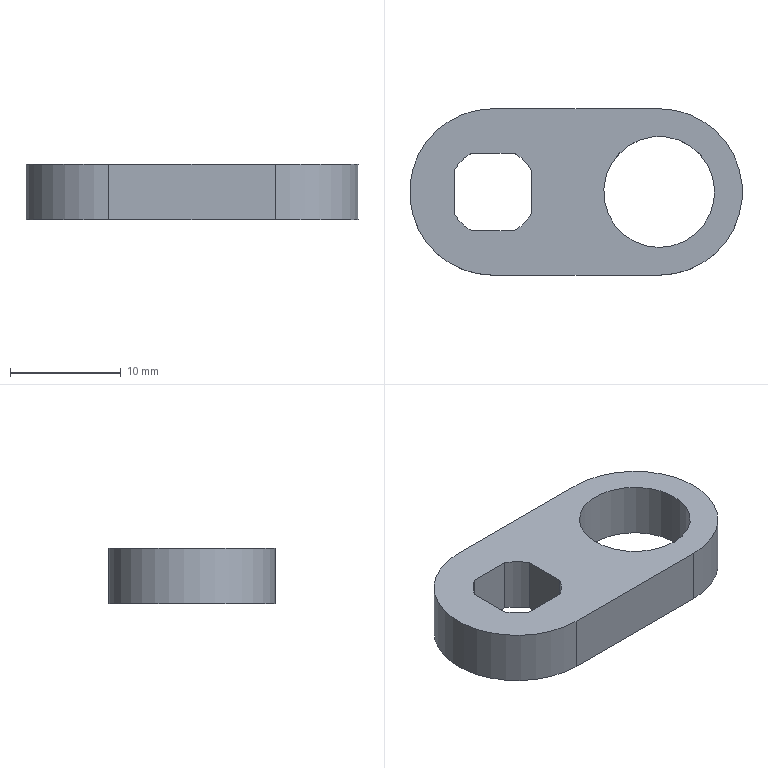Part | NX | features BREP 1, DATUM_CSYS 1 | 1 solid | 15 faces | box 30 x 15 x 5 mm | volume 1391 mm3 | plane 8 | cylinder 7 | commonest cylinder face diameters 8 x4 15 x2 10 x1
STEP:
#1=CARTESIAN_POINT('',(15.,7.5,0.));
#2=VERTEX_POINT('',#1);
#3=CARTESIAN_POINT('',(0.,7.5,0.));
#4=VERTEX_POINT('',#3);
#5=CARTESIAN_POINT('',(15.,7.5,0.));
#6=DIRECTION('',(-1.,0.,0.));
#7=VECTOR('',#6,1000.);
#8=LINE('',#5,#7);
#9=EDGE_CURVE('',#2,#4,#8,.T.);
#10=ORIENTED_EDGE('',*,*,#9,.F.);
#11=CARTESIAN_POINT('',(15.,-7.5,0.));
#12=VERTEX_POINT('',#11);
#13=CARTESIAN_POINT('',(15.,0.,0.));
#14=DIRECTION('',(0.,0.,1.));
#15=DIRECTION('',(0.,-1.,0.));
#16=AXIS2_PLACEMENT_3D('',#13,#14,#15);
#17=CIRCLE('',#16,7.5);
#18=EDGE_CURVE('',#12,#2,#17,.T.);
#19=ORIENTED_EDGE('',*,*,#18,.F.);
#20=CARTESIAN_POINT('',(0.,-7.5,0.));
#21=VERTEX_POINT('',#20);
#22=CARTESIAN_POINT('',(0.,-7.5,0.));
#23=DIRECTION('',(1.,0.,0.));
#24=VECTOR('',#23,1000.);
#25=LINE('',#22,#24);
#26=EDGE_CURVE('',#21,#12,#25,.T.);
#27=ORIENTED_EDGE('',*,*,#26,.F.);
#28=CARTESIAN_POINT('',(0.,0.,0.));
#29=DIRECTION('',(0.,0.,1.));
#30=DIRECTION('',(0.,1.,0.));
#31=AXIS2_PLACEMENT_3D('',#28,#29,#30);
#32=CIRCLE('',#31,7.5);
#33=EDGE_CURVE('',#4,#21,#32,.T.);
#34=ORIENTED_EDGE('',*,*,#33,.F.);
#35=EDGE_LOOP('',(#10,#19,#27,#34));
#36=FACE_BOUND('',#35,.T.);
#37=CARTESIAN_POINT('',(1.936,-3.5,0.));
#38=VERTEX_POINT('',#37);
#39=CARTESIAN_POINT('',(-1.936,-3.5,0.));
#40=VERTEX_POINT('',#39);
#41=CARTESIAN_POINT('',(1.936,-3.5,0.));
#42=DIRECTION('',(-1.,0.,0.));
#43=VECTOR('',#42,1000.);
#44=LINE('',#41,#43);
#45=EDGE_CURVE('',#38,#40,#44,.T.);
#46=ORIENTED_EDGE('',*,*,#45,.F.);
#47=CARTESIAN_POINT('',(3.5,-1.936,0.));
#48=VERTEX_POINT('',#47);
#49=CARTESIAN_POINT('',(0.,0.,0.));
#50=DIRECTION('',(0.,0.,-1.));
#51=DIRECTION('',(0.875,-0.4841,0.));
#52=AXIS2_PLACEMENT_3D('',#49,#50,#51);
#53=CIRCLE('',#52,4.);
#54=EDGE_CURVE('',#48,#38,#53,.T.);
#55=ORIENTED_EDGE('',*,*,#54,.F.);
#56=CARTESIAN_POINT('',(3.5,1.936,0.));
#57=VERTEX_POINT('',#56);
#58=CARTESIAN_POINT('',(3.5,1.936,0.));
#59=DIRECTION('',(0.,-1.,0.));
#60=VECTOR('',#59,1000.);
#61=LINE('',#58,#60);
#62=EDGE_CURVE('',#57,#48,#61,.T.);
#63=ORIENTED_EDGE('',*,*,#62,.F.);
#64=CARTESIAN_POINT('',(1.936,3.5,0.));
#65=VERTEX_POINT('',#64);
#66=CARTESIAN_POINT('',(0.,0.,0.));
#67=DIRECTION('',(0.,0.,-1.));
#68=DIRECTION('',(0.4841,0.875,0.));
#69=AXIS2_PLACEMENT_3D('',#66,#67,#68);
#70=CIRCLE('',#69,4.);
#71=EDGE_CURVE('',#65,#57,#70,.T.);
#72=ORIENTED_EDGE('',*,*,#71,.F.);
#73=CARTESIAN_POINT('',(-1.936,3.5,0.));
#74=VERTEX_POINT('',#73);
#75=CARTESIAN_POINT('',(-1.936,3.5,0.));
#76=DIRECTION('',(1.,0.,0.));
#77=VECTOR('',#76,1000.);
#78=LINE('',#75,#77);
#79=EDGE_CURVE('',#74,#65,#78,.T.);
#80=ORIENTED_EDGE('',*,*,#79,.F.);
#81=CARTESIAN_POINT('',(-3.5,1.936,0.));
#82=VERTEX_POINT('',#81);
#83=CARTESIAN_POINT('',(0.,0.,0.));
#84=DIRECTION('',(0.,0.,-1.));
#85=DIRECTION('',(-0.875,0.4841,0.));
#86=AXIS2_PLACEMENT_3D('',#83,#84,#85);
#87=CIRCLE('',#86,4.);
#88=EDGE_CURVE('',#82,#74,#87,.T.);
#89=ORIENTED_EDGE('',*,*,#88,.F.);
#90=CARTESIAN_POINT('',(-3.5,-1.936,0.));
#91=VERTEX_POINT('',#90);
#92=CARTESIAN_POINT('',(-3.5,-1.936,0.));
#93=DIRECTION('',(0.,1.,0.));
#94=VECTOR('',#93,1000.);
#95=LINE('',#92,#94);
#96=EDGE_CURVE('',#91,#82,#95,.T.);
#97=ORIENTED_EDGE('',*,*,#96,.F.);
#98=CARTESIAN_POINT('',(0.,0.,0.));
#99=DIRECTION('',(0.,0.,-1.));
#100=DIRECTION('',(-0.4841,-0.875,0.));
#101=AXIS2_PLACEMENT_3D('',#98,#99,#100);
#102=CIRCLE('',#101,4.);
#103=EDGE_CURVE('',#40,#91,#102,.T.);
#104=ORIENTED_EDGE('',*,*,#103,.F.);
#105=EDGE_LOOP('',(#46,#55,#63,#72,#80,#89,#97,#104));
#106=FACE_BOUND('',#105,.T.);
#107=CARTESIAN_POINT('',(15.,-5.,0.));
#108=VERTEX_POINT('',#107);
#109=CARTESIAN_POINT('',(15.,0.,0.));
#110=DIRECTION('',(0.,0.,-1.));
#111=DIRECTION('',(0.,-1.,0.));
#112=AXIS2_PLACEMENT_3D('',#109,#110,#111);
#113=CIRCLE('',#112,5.);
#114=EDGE_CURVE('',#108,#108,#113,.T.);
#115=ORIENTED_EDGE('',*,*,#114,.F.);
#116=EDGE_LOOP('',(#115));
#117=FACE_BOUND('',#116,.T.);
#118=CARTESIAN_POINT('',(7.5,7.5,0.));
#119=DIRECTION('',(0.,0.,1.));
#120=DIRECTION('',(-1.,0.,0.));
#121=AXIS2_PLACEMENT_3D('',#118,#119,#120);
#122=PLANE('',#121);
#123=ADVANCED_FACE('',(#36,#106,#117),#122,.F.);
#124=CARTESIAN_POINT('',(0.,7.5,5.));
#125=VERTEX_POINT('',#124);
#126=CARTESIAN_POINT('',(0.,-7.5,5.));
#127=VERTEX_POINT('',#126);
#128=CARTESIAN_POINT('',(0.,0.,5.));
#129=DIRECTION('',(0.,0.,1.));
#130=DIRECTION('',(0.,1.,0.));
#131=AXIS2_PLACEMENT_3D('',#128,#129,#130);
#132=CIRCLE('',#131,7.5);
#133=EDGE_CURVE('',#125,#127,#132,.T.);
#134=ORIENTED_EDGE('',*,*,#133,.T.);
#135=CARTESIAN_POINT('',(15.,-7.5,5.));
#136=VERTEX_POINT('',#135);
#137=CARTESIAN_POINT('',(0.,-7.5,5.));
#138=DIRECTION('',(1.,0.,0.));
#139=VECTOR('',#138,1000.);
#140=LINE('',#137,#139);
#141=EDGE_CURVE('',#127,#136,#140,.T.);
#142=ORIENTED_EDGE('',*,*,#141,.T.);
#143=CARTESIAN_POINT('',(15.,7.5,5.));
#144=VERTEX_POINT('',#143);
#145=CARTESIAN_POINT('',(15.,0.,5.));
#146=DIRECTION('',(0.,0.,1.));
#147=DIRECTION('',(0.,-1.,0.));
#148=AXIS2_PLACEMENT_3D('',#145,#146,#147);
#149=CIRCLE('',#148,7.5);
#150=EDGE_CURVE('',#136,#144,#149,.T.);
#151=ORIENTED_EDGE('',*,*,#150,.T.);
#152=CARTESIAN_POINT('',(15.,7.5,5.));
#153=DIRECTION('',(-1.,0.,0.));
#154=VECTOR('',#153,1000.);
#155=LINE('',#152,#154);
#156=EDGE_CURVE('',#144,#125,#155,.T.);
#157=ORIENTED_EDGE('',*,*,#156,.T.);
#158=EDGE_LOOP('',(#134,#142,#151,#157));
#159=FACE_BOUND('',#158,.T.);
#160=CARTESIAN_POINT('',(-1.936,-3.5,5.));
#161=VERTEX_POINT('',#160);
#162=CARTESIAN_POINT('',(-3.5,-1.936,5.));
#163=VERTEX_POINT('',#162);
#164=CARTESIAN_POINT('',(0.,0.,5.));
#165=DIRECTION('',(0.,0.,-1.));
#166=DIRECTION('',(-0.4841,-0.875,0.));
#167=AXIS2_PLACEMENT_3D('',#164,#165,#166);
#168=CIRCLE('',#167,4.);
#169=EDGE_CURVE('',#161,#163,#168,.T.);
#170=ORIENTED_EDGE('',*,*,#169,.T.);
#171=CARTESIAN_POINT('',(-3.5,1.936,5.));
#172=VERTEX_POINT('',#171);
#173=CARTESIAN_POINT('',(-3.5,-1.936,5.));
#174=DIRECTION('',(0.,1.,0.));
#175=VECTOR('',#174,1000.);
#176=LINE('',#173,#175);
#177=EDGE_CURVE('',#163,#172,#176,.T.);
#178=ORIENTED_EDGE('',*,*,#177,.T.);
#179=CARTESIAN_POINT('',(-1.936,3.5,5.));
#180=VERTEX_POINT('',#179);
#181=CARTESIAN_POINT('',(0.,0.,5.));
#182=DIRECTION('',(0.,0.,-1.));
#183=DIRECTION('',(-0.875,0.4841,0.));
#184=AXIS2_PLACEMENT_3D('',#181,#182,#183);
#185=CIRCLE('',#184,4.);
#186=EDGE_CURVE('',#172,#180,#185,.T.);
#187=ORIENTED_EDGE('',*,*,#186,.T.);
#188=CARTESIAN_POINT('',(1.936,3.5,5.));
#189=VERTEX_POINT('',#188);
#190=CARTESIAN_POINT('',(-1.936,3.5,5.));
#191=DIRECTION('',(1.,0.,0.));
#192=VECTOR('',#191,1000.);
#193=LINE('',#190,#192);
#194=EDGE_CURVE('',#180,#189,#193,.T.);
#195=ORIENTED_EDGE('',*,*,#194,.T.);
#196=CARTESIAN_POINT('',(3.5,1.936,5.));
#197=VERTEX_POINT('',#196);
#198=CARTESIAN_POINT('',(0.,0.,5.));
#199=DIRECTION('',(0.,0.,-1.));
#200=DIRECTION('',(0.4841,0.875,0.));
#201=AXIS2_PLACEMENT_3D('',#198,#199,#200);
#202=CIRCLE('',#201,4.);
#203=EDGE_CURVE('',#189,#197,#202,.T.);
#204=ORIENTED_EDGE('',*,*,#203,.T.);
#205=CARTESIAN_POINT('',(3.5,-1.936,5.));
#206=VERTEX_POINT('',#205);
#207=CARTESIAN_POINT('',(3.5,1.936,5.));
#208=DIRECTION('',(0.,-1.,0.));
#209=VECTOR('',#208,1000.);
#210=LINE('',#207,#209);
#211=EDGE_CURVE('',#197,#206,#210,.T.);
#212=ORIENTED_EDGE('',*,*,#211,.T.);
#213=CARTESIAN_POINT('',(1.936,-3.5,5.));
#214=VERTEX_POINT('',#213);
#215=CARTESIAN_POINT('',(0.,0.,5.));
#216=DIRECTION('',(0.,0.,-1.));
#217=DIRECTION('',(0.875,-0.4841,0.));
#218=AXIS2_PLACEMENT_3D('',#215,#216,#217);
#219=CIRCLE('',#218,4.);
#220=EDGE_CURVE('',#206,#214,#219,.T.);
#221=ORIENTED_EDGE('',*,*,#220,.T.);
#222=CARTESIAN_POINT('',(1.936,-3.5,5.));
#223=DIRECTION('',(-1.,0.,0.));
#224=VECTOR('',#223,1000.);
#225=LINE('',#222,#224);
#226=EDGE_CURVE('',#214,#161,#225,.T.);
#227=ORIENTED_EDGE('',*,*,#226,.T.);
#228=EDGE_LOOP('',(#170,#178,#187,#195,#204,#212,#221,#227));
#229=FACE_BOUND('',#228,.T.);
#230=CARTESIAN_POINT('',(15.,-5.,5.));
#231=VERTEX_POINT('',#230);
#232=CARTESIAN_POINT('',(15.,0.,5.));
#233=DIRECTION('',(0.,0.,-1.));
#234=DIRECTION('',(0.,-1.,0.));
#235=AXIS2_PLACEMENT_3D('',#232,#233,#234);
#236=CIRCLE('',#235,5.);
#237=EDGE_CURVE('',#231,#231,#236,.T.);
#238=ORIENTED_EDGE('',*,*,#237,.T.);
#239=EDGE_LOOP('',(#238));
#240=FACE_BOUND('',#239,.T.);
#241=CARTESIAN_POINT('',(7.5,7.5,5.));
#242=DIRECTION('',(0.,0.,1.));
#243=DIRECTION('',(-1.,0.,0.));
#244=AXIS2_PLACEMENT_3D('',#241,#242,#243);
#245=PLANE('',#244);
#246=ADVANCED_FACE('',(#159,#229,#240),#245,.T.);
#247=ORIENTED_EDGE('',*,*,#33,.T.);
#248=CARTESIAN_POINT('',(0.,-7.5,0.));
#249=DIRECTION('',(0.,0.,1.));
#250=VECTOR('',#249,1000.);
#251=LINE('',#248,#250);
#252=EDGE_CURVE('',#21,#127,#251,.T.);
#253=ORIENTED_EDGE('',*,*,#252,.T.);
#254=ORIENTED_EDGE('',*,*,#133,.F.);
#255=CARTESIAN_POINT('',(0.,7.5,0.));
#256=DIRECTION('',(0.,0.,1.));
#257=VECTOR('',#256,1000.);
#258=LINE('',#255,#257);
#259=EDGE_CURVE('',#4,#125,#258,.T.);
#260=ORIENTED_EDGE('',*,*,#259,.F.);
#261=EDGE_LOOP('',(#247,#253,#254,#260));
#262=FACE_BOUND('',#261,.T.);
#263=CARTESIAN_POINT('',(0.,0.,0.));
#264=DIRECTION('',(0.,0.,1.));
#265=DIRECTION('',(0.,-1.,0.));
#266=AXIS2_PLACEMENT_3D('',#263,#264,#265);
#267=CYLINDRICAL_SURFACE('',#266,7.5);
#268=ADVANCED_FACE('',(#262),#267,.T.);
#269=ORIENTED_EDGE('',*,*,#26,.T.);
#270=CARTESIAN_POINT('',(15.,-7.5,0.));
#271=DIRECTION('',(0.,0.,1.));
#272=VECTOR('',#271,1000.);
#273=LINE('',#270,#272);
#274=EDGE_CURVE('',#12,#136,#273,.T.);
#275=ORIENTED_EDGE('',*,*,#274,.T.);
#276=ORIENTED_EDGE('',*,*,#141,.F.);
#277=ORIENTED_EDGE('',*,*,#252,.F.);
#278=EDGE_LOOP('',(#269,#275,#276,#277));
#279=FACE_BOUND('',#278,.T.);
#280=CARTESIAN_POINT('',(7.5,-7.5,2.5));
#281=DIRECTION('',(0.,-1.,0.));
#282=DIRECTION('',(-1.,0.,0.));
#283=AXIS2_PLACEMENT_3D('',#280,#281,#282);
#284=PLANE('',#283);
#285=ADVANCED_FACE('',(#279),#284,.T.);
#286=ORIENTED_EDGE('',*,*,#18,.T.);
#287=CARTESIAN_POINT('',(15.,7.5,0.));
#288=DIRECTION('',(0.,0.,1.));
#289=VECTOR('',#288,1000.);
#290=LINE('',#287,#289);
#291=EDGE_CURVE('',#2,#144,#290,.T.);
#292=ORIENTED_EDGE('',*,*,#291,.T.);
#293=ORIENTED_EDGE('',*,*,#150,.F.);
#294=ORIENTED_EDGE('',*,*,#274,.F.);
#295=EDGE_LOOP('',(#286,#292,#293,#294));
#296=FACE_BOUND('',#295,.T.);
#297=CARTESIAN_POINT('',(15.,0.,0.));
#298=DIRECTION('',(0.,0.,1.));
#299=DIRECTION('',(0.,1.,0.));
#300=AXIS2_PLACEMENT_3D('',#297,#298,#299);
#301=CYLINDRICAL_SURFACE('',#300,7.5);
#302=ADVANCED_FACE('',(#296),#301,.T.);
#303=ORIENTED_EDGE('',*,*,#9,.T.);
#304=ORIENTED_EDGE('',*,*,#259,.T.);
#305=ORIENTED_EDGE('',*,*,#156,.F.);
#306=ORIENTED_EDGE('',*,*,#291,.F.);
#307=EDGE_LOOP('',(#303,#304,#305,#306));
#308=FACE_BOUND('',#307,.T.);
#309=CARTESIAN_POINT('',(7.5,7.5,2.5));
#310=DIRECTION('',(0.,1.,0.));
#311=DIRECTION('',(1.,0.,0.));
#312=AXIS2_PLACEMENT_3D('',#309,#310,#311);
#313=PLANE('',#312);
#314=ADVANCED_FACE('',(#308),#313,.T.);
#315=CARTESIAN_POINT('',(15.,-5.,5.));
#316=DIRECTION('',(0.,0.,-1.));
#317=VECTOR('',#316,1000.);
#318=LINE('',#315,#317);
#319=EDGE_CURVE('',#231,#108,#318,.T.);
#320=ORIENTED_EDGE('',*,*,#319,.T.);
#321=ORIENTED_EDGE('',*,*,#114,.T.);
#322=ORIENTED_EDGE('',*,*,#319,.F.);
#323=ORIENTED_EDGE('',*,*,#237,.F.);
#324=EDGE_LOOP('',(#320,#321,#322,#323));
#325=FACE_BOUND('',#324,.T.);
#326=CARTESIAN_POINT('',(15.,0.,5.));
#327=DIRECTION('',(0.,0.,-1.));
#328=DIRECTION('',(0.,1.,0.));
#329=AXIS2_PLACEMENT_3D('',#326,#327,#328);
#330=CYLINDRICAL_SURFACE('',#329,5.);
#331=ADVANCED_FACE('',(#325),#330,.F.);
#332=CARTESIAN_POINT('',(-3.5,-1.936,5.));
#333=DIRECTION('',(0.,0.,-1.));
#334=VECTOR('',#333,1000.);
#335=LINE('',#332,#334);
#336=EDGE_CURVE('',#163,#91,#335,.T.);
#337=ORIENTED_EDGE('',*,*,#336,.F.);
#338=ORIENTED_EDGE('',*,*,#169,.F.);
#339=CARTESIAN_POINT('',(-1.936,-3.5,5.));
#340=DIRECTION('',(0.,0.,-1.));
#341=VECTOR('',#340,1000.);
#342=LINE('',#339,#341);
#343=EDGE_CURVE('',#161,#40,#342,.T.);
#344=ORIENTED_EDGE('',*,*,#343,.T.);
#345=ORIENTED_EDGE('',*,*,#103,.T.);
#346=EDGE_LOOP('',(#337,#338,#344,#345));
#347=FACE_BOUND('',#346,.T.);
#348=CARTESIAN_POINT('',(0.,0.,5.));
#349=DIRECTION('',(0.,0.,-1.));
#350=DIRECTION('',(-0.4841,-0.875,0.));
#351=AXIS2_PLACEMENT_3D('',#348,#349,#350);
#352=CYLINDRICAL_SURFACE('',#351,4.);
#353=ADVANCED_FACE('',(#347),#352,.F.);
#354=CARTESIAN_POINT('',(-1.936,3.5,5.));
#355=DIRECTION('',(0.,0.,-1.));
#356=VECTOR('',#355,1000.);
#357=LINE('',#354,#356);
#358=EDGE_CURVE('',#180,#74,#357,.T.);
#359=ORIENTED_EDGE('',*,*,#358,.F.);
#360=ORIENTED_EDGE('',*,*,#186,.F.);
#361=CARTESIAN_POINT('',(-3.5,1.936,5.));
#362=DIRECTION('',(0.,0.,-1.));
#363=VECTOR('',#362,1000.);
#364=LINE('',#361,#363);
#365=EDGE_CURVE('',#172,#82,#364,.T.);
#366=ORIENTED_EDGE('',*,*,#365,.T.);
#367=ORIENTED_EDGE('',*,*,#88,.T.);
#368=EDGE_LOOP('',(#359,#360,#366,#367));
#369=FACE_BOUND('',#368,.T.);
#370=CARTESIAN_POINT('',(0.,0.,5.));
#371=DIRECTION('',(0.,0.,-1.));
#372=DIRECTION('',(-0.4841,-0.875,0.));
#373=AXIS2_PLACEMENT_3D('',#370,#371,#372);
#374=CYLINDRICAL_SURFACE('',#373,4.);
#375=ADVANCED_FACE('',(#369),#374,.F.);
#376=CARTESIAN_POINT('',(1.936,-3.5,5.));
#377=DIRECTION('',(0.,0.,-1.));
#378=VECTOR('',#377,1000.);
#379=LINE('',#376,#378);
#380=EDGE_CURVE('',#214,#38,#379,.T.);
#381=ORIENTED_EDGE('',*,*,#380,.F.);
#382=ORIENTED_EDGE('',*,*,#220,.F.);
#383=CARTESIAN_POINT('',(3.5,-1.936,5.));
#384=DIRECTION('',(0.,0.,-1.));
#385=VECTOR('',#384,1000.);
#386=LINE('',#383,#385);
#387=EDGE_CURVE('',#206,#48,#386,.T.);
#388=ORIENTED_EDGE('',*,*,#387,.T.);
#389=ORIENTED_EDGE('',*,*,#54,.T.);
#390=EDGE_LOOP('',(#381,#382,#388,#389));
#391=FACE_BOUND('',#390,.T.);
#392=CARTESIAN_POINT('',(0.,0.,5.));
#393=DIRECTION('',(0.,0.,-1.));
#394=DIRECTION('',(-0.4841,-0.875,0.));
#395=AXIS2_PLACEMENT_3D('',#392,#393,#394);
#396=CYLINDRICAL_SURFACE('',#395,4.);
#397=ADVANCED_FACE('',(#391),#396,.F.);
#398=CARTESIAN_POINT('',(3.5,1.936,5.));
#399=DIRECTION('',(0.,0.,-1.));
#400=VECTOR('',#399,1000.);
#401=LINE('',#398,#400);
#402=EDGE_CURVE('',#197,#57,#401,.T.);
#403=ORIENTED_EDGE('',*,*,#402,.F.);
#404=ORIENTED_EDGE('',*,*,#203,.F.);
#405=CARTESIAN_POINT('',(1.936,3.5,5.));
#406=DIRECTION('',(0.,0.,-1.));
#407=VECTOR('',#406,1000.);
#408=LINE('',#405,#407);
#409=EDGE_CURVE('',#189,#65,#408,.T.);
#410=ORIENTED_EDGE('',*,*,#409,.T.);
#411=ORIENTED_EDGE('',*,*,#71,.T.);
#412=EDGE_LOOP('',(#403,#404,#410,#411));
#413=FACE_BOUND('',#412,.T.);
#414=CARTESIAN_POINT('',(0.,0.,5.));
#415=DIRECTION('',(0.,0.,-1.));
#416=DIRECTION('',(-0.4841,-0.875,0.));
#417=AXIS2_PLACEMENT_3D('',#414,#415,#416);
#418=CYLINDRICAL_SURFACE('',#417,4.);
#419=ADVANCED_FACE('',(#413),#418,.F.);
#420=ORIENTED_EDGE('',*,*,#358,.T.);
#421=ORIENTED_EDGE('',*,*,#79,.T.);
#422=ORIENTED_EDGE('',*,*,#409,.F.);
#423=ORIENTED_EDGE('',*,*,#194,.F.);
#424=EDGE_LOOP('',(#420,#421,#422,#423));
#425=FACE_BOUND('',#424,.T.);
#426=CARTESIAN_POINT('',(0.,3.5,2.5));
#427=DIRECTION('',(0.,1.,0.));
#428=DIRECTION('',(-1.,0.,0.));
#429=AXIS2_PLACEMENT_3D('',#426,#427,#428);
#430=PLANE('',#429);
#431=ADVANCED_FACE('',(#425),#430,.F.);
#432=ORIENTED_EDGE('',*,*,#336,.T.);
#433=ORIENTED_EDGE('',*,*,#96,.T.);
#434=ORIENTED_EDGE('',*,*,#365,.F.);
#435=ORIENTED_EDGE('',*,*,#177,.F.);
#436=EDGE_LOOP('',(#432,#433,#434,#435));
#437=FACE_BOUND('',#436,.T.);
#438=CARTESIAN_POINT('',(-3.5,0.,2.5));
#439=DIRECTION('',(-1.,0.,0.));
#440=DIRECTION('',(0.,-1.,0.));
#441=AXIS2_PLACEMENT_3D('',#438,#439,#440);
#442=PLANE('',#441);
#443=ADVANCED_FACE('',(#437),#442,.F.);
#444=ORIENTED_EDGE('',*,*,#402,.T.);
#445=ORIENTED_EDGE('',*,*,#62,.T.);
#446=ORIENTED_EDGE('',*,*,#387,.F.);
#447=ORIENTED_EDGE('',*,*,#211,.F.);
#448=EDGE_LOOP('',(#444,#445,#446,#447));
#449=FACE_BOUND('',#448,.T.);
#450=CARTESIAN_POINT('',(3.5,0.,2.5));
#451=DIRECTION('',(1.,0.,0.));
#452=DIRECTION('',(0.,1.,0.));
#453=AXIS2_PLACEMENT_3D('',#450,#451,#452);
#454=PLANE('',#453);
#455=ADVANCED_FACE('',(#449),#454,.F.);
#456=ORIENTED_EDGE('',*,*,#380,.T.);
#457=ORIENTED_EDGE('',*,*,#45,.T.);
#458=ORIENTED_EDGE('',*,*,#343,.F.);
#459=ORIENTED_EDGE('',*,*,#226,.F.);
#460=EDGE_LOOP('',(#456,#457,#458,#459));
#461=FACE_BOUND('',#460,.T.);
#462=CARTESIAN_POINT('',(0.,-3.5,2.5));
#463=DIRECTION('',(0.,-1.,0.));
#464=DIRECTION('',(1.,0.,0.));
#465=AXIS2_PLACEMENT_3D('',#462,#463,#464);
#466=PLANE('',#465);
#467=ADVANCED_FACE('',(#461),#466,.F.);
#468=CLOSED_SHELL('',(#123,#246,#268,#285,#302,#314,#331,#353,#375,#397,#419,#431,#443,#455,#467));
#469=MANIFOLD_SOLID_BREP('',#468);
#470=(LENGTH_UNIT()NAMED_UNIT(*)SI_UNIT(.MILLI.,.METRE.));
#471=UNCERTAINTY_MEASURE_WITH_UNIT(LENGTH_MEASURE(0.00001),#470,'','');
#472=(NAMED_UNIT(*)PLANE_ANGLE_UNIT()SI_UNIT($,.RADIAN.));
#473=(NAMED_UNIT(*)SI_UNIT($,.STERADIAN.)SOLID_ANGLE_UNIT());
#474=(GEOMETRIC_REPRESENTATION_CONTEXT(3)GLOBAL_UNCERTAINTY_ASSIGNED_CONTEXT((#471))GLOBAL_UNIT_ASSIGNED_CONTEXT((#470,#472,#473))REPRESENTATION_CONTEXT('',''));
#475=ADVANCED_BREP_SHAPE_REPRESENTATION('',(#469),#474);